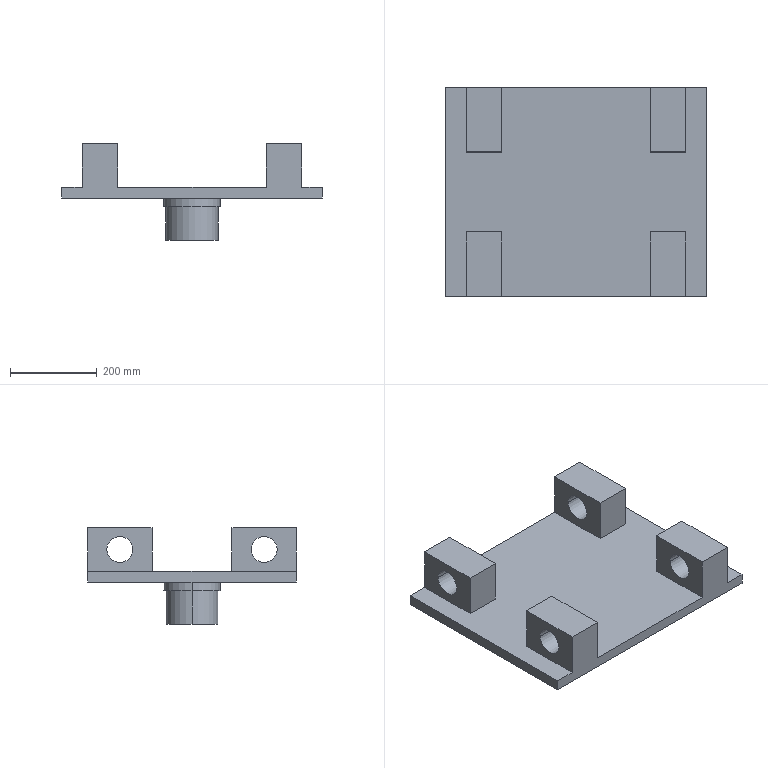Part | SolidWorks | features ICE 5, Extrusion 1 | 1 solid | 39 faces | box 600 x 480 x 222 mm | volume 11838573 mm3 | plane 25 | cylinder 14 | commonest cylinder face diameters 60 x8 80 x2 120 x2 130 x2
STEP:
#1=CARTESIAN_POINT('',(340.,240.,-97.));
#2=VERTEX_POINT('',#1);
#3=CARTESIAN_POINT('',(260.,240.,-97.));
#4=VERTEX_POINT('',#3);
#5=CARTESIAN_POINT('',(300.,240.,-97.));
#6=DIRECTION('',(0.,0.,-1.));
#7=DIRECTION('',(-1.,0.,0.));
#8=AXIS2_PLACEMENT_3D('',#5,#6,#7);
#9=CIRCLE('',#8,40.);
#10=EDGE_CURVE('',#2,#4,#9,.T.);
#11=ORIENTED_EDGE('',*,*,#10,.T.);
#12=CARTESIAN_POINT('',(260.,240.,-12.5));
#13=VERTEX_POINT('',#12);
#14=CARTESIAN_POINT('',(260.,240.,-20.));
#15=DIRECTION('',(0.,0.,1.));
#16=VECTOR('',#15,1000.);
#17=LINE('',#14,#16);
#18=EDGE_CURVE('',#4,#13,#17,.T.);
#19=ORIENTED_EDGE('',*,*,#18,.T.);
#20=CARTESIAN_POINT('',(340.,240.,-12.5));
#21=VERTEX_POINT('',#20);
#22=CARTESIAN_POINT('',(300.,240.,-12.5));
#23=DIRECTION('',(0.,0.,-1.));
#24=DIRECTION('',(-1.,0.,0.));
#25=AXIS2_PLACEMENT_3D('',#22,#23,#24);
#26=CIRCLE('',#25,40.);
#27=EDGE_CURVE('',#21,#13,#26,.T.);
#28=ORIENTED_EDGE('',*,*,#27,.F.);
#29=CARTESIAN_POINT('',(340.,240.,-20.));
#30=DIRECTION('',(0.,0.,1.));
#31=VECTOR('',#30,1000.);
#32=LINE('',#29,#31);
#33=EDGE_CURVE('',#2,#21,#32,.T.);
#34=ORIENTED_EDGE('',*,*,#33,.F.);
#35=EDGE_LOOP('',(#11,#19,#28,#34));
#36=FACE_OUTER_BOUND('',#35,.T.);
#37=CARTESIAN_POINT('',(300.,240.,-20.));
#38=DIRECTION('',(0.,0.,1.));
#39=DIRECTION('',(1.,0.,0.));
#40=AXIS2_PLACEMENT_3D('',#37,#38,#39);
#41=CYLINDRICAL_SURFACE('',#40,40.);
#42=ADVANCED_FACE('',(#36),#41,.F.);
#43=CARTESIAN_POINT('',(240.,240.,-97.));
#44=VERTEX_POINT('',#43);
#45=CARTESIAN_POINT('',(360.,240.,-97.));
#46=VERTEX_POINT('',#45);
#47=CARTESIAN_POINT('',(300.,240.,-97.));
#48=DIRECTION('',(0.,0.,-1.));
#49=DIRECTION('',(-1.,0.,0.));
#50=AXIS2_PLACEMENT_3D('',#47,#48,#49);
#51=CIRCLE('',#50,60.);
#52=EDGE_CURVE('',#44,#46,#51,.T.);
#53=ORIENTED_EDGE('',*,*,#52,.F.);
#54=CARTESIAN_POINT('',(240.,240.,-20.));
#55=VERTEX_POINT('',#54);
#56=CARTESIAN_POINT('',(240.,240.,-97.));
#57=DIRECTION('',(0.,0.,1.));
#58=VECTOR('',#57,1000.);
#59=LINE('',#56,#58);
#60=EDGE_CURVE('',#44,#55,#59,.T.);
#61=ORIENTED_EDGE('',*,*,#60,.T.);
#62=CARTESIAN_POINT('',(360.,240.,-20.));
#63=VERTEX_POINT('',#62);
#64=CARTESIAN_POINT('',(300.,240.,-20.));
#65=DIRECTION('',(0.,0.,-1.));
#66=DIRECTION('',(-1.,0.,0.));
#67=AXIS2_PLACEMENT_3D('',#64,#65,#66);
#68=CIRCLE('',#67,60.);
#69=EDGE_CURVE('',#55,#63,#68,.T.);
#70=ORIENTED_EDGE('',*,*,#69,.T.);
#71=CARTESIAN_POINT('',(360.,240.,-97.));
#72=DIRECTION('',(0.,0.,1.));
#73=VECTOR('',#72,1000.);
#74=LINE('',#71,#73);
#75=EDGE_CURVE('',#46,#63,#74,.T.);
#76=ORIENTED_EDGE('',*,*,#75,.F.);
#77=EDGE_LOOP('',(#53,#61,#70,#76));
#78=FACE_OUTER_BOUND('',#77,.T.);
#79=CARTESIAN_POINT('',(300.,240.,-97.));
#80=DIRECTION('',(0.,0.,1.));
#81=DIRECTION('',(1.,0.,0.));
#82=AXIS2_PLACEMENT_3D('',#79,#80,#81);
#83=CYLINDRICAL_SURFACE('',#82,60.);
#84=ADVANCED_FACE('',(#78),#83,.T.);
#85=CARTESIAN_POINT('',(235.,240.,-20.));
#86=VERTEX_POINT('',#85);
#87=CARTESIAN_POINT('',(365.,240.,-20.));
#88=VERTEX_POINT('',#87);
#89=CARTESIAN_POINT('',(300.,240.,-20.));
#90=DIRECTION('',(0.,0.,-1.));
#91=DIRECTION('',(-1.,0.,0.));
#92=AXIS2_PLACEMENT_3D('',#89,#90,#91);
#93=CIRCLE('',#92,65.);
#94=EDGE_CURVE('',#86,#88,#93,.T.);
#95=ORIENTED_EDGE('',*,*,#94,.F.);
#96=CARTESIAN_POINT('',(235.,240.,0.));
#97=VERTEX_POINT('',#96);
#98=CARTESIAN_POINT('',(235.,240.,-20.));
#99=DIRECTION('',(0.,0.,1.));
#100=VECTOR('',#99,1000.);
#101=LINE('',#98,#100);
#102=EDGE_CURVE('',#86,#97,#101,.T.);
#103=ORIENTED_EDGE('',*,*,#102,.T.);
#104=CARTESIAN_POINT('',(365.,240.,0.));
#105=VERTEX_POINT('',#104);
#106=CARTESIAN_POINT('',(300.,240.,0.));
#107=DIRECTION('',(0.,0.,-1.));
#108=DIRECTION('',(-1.,0.,0.));
#109=AXIS2_PLACEMENT_3D('',#106,#107,#108);
#110=CIRCLE('',#109,65.);
#111=EDGE_CURVE('',#97,#105,#110,.T.);
#112=ORIENTED_EDGE('',*,*,#111,.T.);
#113=CARTESIAN_POINT('',(365.,240.,-20.));
#114=DIRECTION('',(0.,0.,1.));
#115=VECTOR('',#114,1000.);
#116=LINE('',#113,#115);
#117=EDGE_CURVE('',#88,#105,#116,.T.);
#118=ORIENTED_EDGE('',*,*,#117,.F.);
#119=EDGE_LOOP('',(#95,#103,#112,#118));
#120=FACE_OUTER_BOUND('',#119,.T.);
#121=CARTESIAN_POINT('',(300.,240.,-20.));
#122=DIRECTION('',(0.,0.,1.));
#123=DIRECTION('',(1.,0.,0.));
#124=AXIS2_PLACEMENT_3D('',#121,#122,#123);
#125=CYLINDRICAL_SURFACE('',#124,65.);
#126=ADVANCED_FACE('',(#120),#125,.T.);
#127=CARTESIAN_POINT('',(129.5,44.,75.));
#128=VERTEX_POINT('',#127);
#129=CARTESIAN_POINT('',(129.5,104.,75.));
#130=VERTEX_POINT('',#129);
#131=CARTESIAN_POINT('',(129.5,74.,75.));
#132=DIRECTION('',(1.,0.,0.));
#133=DIRECTION('',(0.,0.,-1.));
#134=AXIS2_PLACEMENT_3D('',#131,#132,#133);
#135=CIRCLE('',#134,30.);
#136=EDGE_CURVE('',#128,#130,#135,.T.);
#137=ORIENTED_EDGE('',*,*,#136,.T.);
#138=CARTESIAN_POINT('',(47.5,104.,75.));
#139=VERTEX_POINT('',#138);
#140=CARTESIAN_POINT('',(600.,104.,75.));
#141=DIRECTION('',(-1.,0.,0.));
#142=VECTOR('',#141,1000.);
#143=LINE('',#140,#142);
#144=EDGE_CURVE('',#130,#139,#143,.T.);
#145=ORIENTED_EDGE('',*,*,#144,.T.);
#146=CARTESIAN_POINT('',(47.5,44.,75.));
#147=VERTEX_POINT('',#146);
#148=CARTESIAN_POINT('',(47.5,74.,75.));
#149=DIRECTION('',(-1.,0.,0.));
#150=DIRECTION('',(0.,-1.,0.));
#151=AXIS2_PLACEMENT_3D('',#148,#149,#150);
#152=CIRCLE('',#151,30.);
#153=EDGE_CURVE('',#139,#147,#152,.T.);
#154=ORIENTED_EDGE('',*,*,#153,.T.);
#155=CARTESIAN_POINT('',(600.,44.,75.));
#156=DIRECTION('',(-1.,0.,0.));
#157=VECTOR('',#156,1000.);
#158=LINE('',#155,#157);
#159=EDGE_CURVE('',#128,#147,#158,.T.);
#160=ORIENTED_EDGE('',*,*,#159,.F.);
#161=EDGE_LOOP('',(#137,#145,#154,#160));
#162=FACE_OUTER_BOUND('',#161,.T.);
#163=CARTESIAN_POINT('',(600.,74.,75.));
#164=DIRECTION('',(-1.,0.,0.));
#165=DIRECTION('',(0.,-1.,0.));
#166=AXIS2_PLACEMENT_3D('',#163,#164,#165);
#167=CYLINDRICAL_SURFACE('',#166,30.);
#168=ADVANCED_FACE('',(#162),#167,.F.);
#169=CARTESIAN_POINT('',(552.5,44.,75.));
#170=VERTEX_POINT('',#169);
#171=CARTESIAN_POINT('',(552.5,104.,75.));
#172=VERTEX_POINT('',#171);
#173=CARTESIAN_POINT('',(552.5,74.,75.));
#174=DIRECTION('',(1.,0.,0.));
#175=DIRECTION('',(0.,1.,0.));
#176=AXIS2_PLACEMENT_3D('',#173,#174,#175);
#177=CIRCLE('',#176,30.);
#178=EDGE_CURVE('',#170,#172,#177,.T.);
#179=ORIENTED_EDGE('',*,*,#178,.T.);
#180=CARTESIAN_POINT('',(470.5,104.,75.));
#181=VERTEX_POINT('',#180);
#182=CARTESIAN_POINT('',(600.,104.,75.));
#183=DIRECTION('',(-1.,0.,0.));
#184=VECTOR('',#183,1000.);
#185=LINE('',#182,#184);
#186=EDGE_CURVE('',#172,#181,#185,.T.);
#187=ORIENTED_EDGE('',*,*,#186,.T.);
#188=CARTESIAN_POINT('',(470.5,44.,75.));
#189=VERTEX_POINT('',#188);
#190=CARTESIAN_POINT('',(470.5,74.,75.));
#191=DIRECTION('',(1.,0.,0.));
#192=DIRECTION('',(0.,0.,-1.));
#193=AXIS2_PLACEMENT_3D('',#190,#191,#192);
#194=CIRCLE('',#193,30.);
#195=EDGE_CURVE('',#189,#181,#194,.T.);
#196=ORIENTED_EDGE('',*,*,#195,.F.);
#197=CARTESIAN_POINT('',(600.,44.,75.));
#198=DIRECTION('',(-1.,0.,0.));
#199=VECTOR('',#198,1000.);
#200=LINE('',#197,#199);
#201=EDGE_CURVE('',#170,#189,#200,.T.);
#202=ORIENTED_EDGE('',*,*,#201,.F.);
#203=EDGE_LOOP('',(#179,#187,#196,#202));
#204=FACE_OUTER_BOUND('',#203,.T.);
#205=CARTESIAN_POINT('',(600.,74.,75.));
#206=DIRECTION('',(-1.,0.,0.));
#207=DIRECTION('',(0.,-1.,0.));
#208=AXIS2_PLACEMENT_3D('',#205,#206,#207);
#209=CYLINDRICAL_SURFACE('',#208,30.);
#210=ADVANCED_FACE('',(#204),#209,.F.);
#211=CARTESIAN_POINT('',(129.5,376.,75.));
#212=VERTEX_POINT('',#211);
#213=CARTESIAN_POINT('',(129.5,436.,75.));
#214=VERTEX_POINT('',#213);
#215=CARTESIAN_POINT('',(129.5,406.,75.));
#216=DIRECTION('',(1.,0.,0.));
#217=DIRECTION('',(0.,1.,0.));
#218=AXIS2_PLACEMENT_3D('',#215,#216,#217);
#219=CIRCLE('',#218,30.);
#220=EDGE_CURVE('',#212,#214,#219,.T.);
#221=ORIENTED_EDGE('',*,*,#220,.T.);
#222=CARTESIAN_POINT('',(47.5,436.,75.));
#223=VERTEX_POINT('',#222);
#224=CARTESIAN_POINT('',(600.,436.,75.));
#225=DIRECTION('',(-1.,0.,0.));
#226=VECTOR('',#225,1000.);
#227=LINE('',#224,#226);
#228=EDGE_CURVE('',#214,#223,#227,.T.);
#229=ORIENTED_EDGE('',*,*,#228,.T.);
#230=CARTESIAN_POINT('',(47.5,376.,75.));
#231=VERTEX_POINT('',#230);
#232=CARTESIAN_POINT('',(47.5,406.,75.));
#233=DIRECTION('',(-1.,0.,0.));
#234=DIRECTION('',(0.,-1.,0.));
#235=AXIS2_PLACEMENT_3D('',#232,#233,#234);
#236=CIRCLE('',#235,30.);
#237=EDGE_CURVE('',#223,#231,#236,.T.);
#238=ORIENTED_EDGE('',*,*,#237,.T.);
#239=CARTESIAN_POINT('',(600.,376.,75.));
#240=DIRECTION('',(-1.,0.,0.));
#241=VECTOR('',#240,1000.);
#242=LINE('',#239,#241);
#243=EDGE_CURVE('',#212,#231,#242,.T.);
#244=ORIENTED_EDGE('',*,*,#243,.F.);
#245=EDGE_LOOP('',(#221,#229,#238,#244));
#246=FACE_OUTER_BOUND('',#245,.T.);
#247=CARTESIAN_POINT('',(600.,406.,75.));
#248=DIRECTION('',(-1.,0.,0.));
#249=DIRECTION('',(0.,-1.,0.));
#250=AXIS2_PLACEMENT_3D('',#247,#248,#249);
#251=CYLINDRICAL_SURFACE('',#250,30.);
#252=ADVANCED_FACE('',(#246),#251,.F.);
#253=CARTESIAN_POINT('',(552.5,376.,75.));
#254=VERTEX_POINT('',#253);
#255=CARTESIAN_POINT('',(552.5,436.,75.));
#256=VERTEX_POINT('',#255);
#257=CARTESIAN_POINT('',(552.5,406.,75.));
#258=DIRECTION('',(1.,0.,0.));
#259=DIRECTION('',(0.,0.,-1.));
#260=AXIS2_PLACEMENT_3D('',#257,#258,#259);
#261=CIRCLE('',#260,30.);
#262=EDGE_CURVE('',#254,#256,#261,.T.);
#263=ORIENTED_EDGE('',*,*,#262,.T.);
#264=CARTESIAN_POINT('',(470.5,436.,75.));
#265=VERTEX_POINT('',#264);
#266=CARTESIAN_POINT('',(600.,436.,75.));
#267=DIRECTION('',(-1.,0.,0.));
#268=VECTOR('',#267,1000.);
#269=LINE('',#266,#268);
#270=EDGE_CURVE('',#256,#265,#269,.T.);
#271=ORIENTED_EDGE('',*,*,#270,.T.);
#272=CARTESIAN_POINT('',(470.5,376.,75.));
#273=VERTEX_POINT('',#272);
#274=CARTESIAN_POINT('',(470.5,406.,75.));
#275=DIRECTION('',(1.,0.,0.));
#276=DIRECTION('',(0.,0.,-1.));
#277=AXIS2_PLACEMENT_3D('',#274,#275,#276);
#278=CIRCLE('',#277,30.);
#279=EDGE_CURVE('',#273,#265,#278,.T.);
#280=ORIENTED_EDGE('',*,*,#279,.F.);
#281=CARTESIAN_POINT('',(600.,376.,75.));
#282=DIRECTION('',(-1.,0.,0.));
#283=VECTOR('',#282,1000.);
#284=LINE('',#281,#283);
#285=EDGE_CURVE('',#254,#273,#284,.T.);
#286=ORIENTED_EDGE('',*,*,#285,.F.);
#287=EDGE_LOOP('',(#263,#271,#280,#286));
#288=FACE_OUTER_BOUND('',#287,.T.);
#289=CARTESIAN_POINT('',(600.,406.,75.));
#290=DIRECTION('',(-1.,0.,0.));
#291=DIRECTION('',(0.,-1.,0.));
#292=AXIS2_PLACEMENT_3D('',#289,#290,#291);
#293=CYLINDRICAL_SURFACE('',#292,30.);
#294=ADVANCED_FACE('',(#288),#293,.F.);
#295=CARTESIAN_POINT('',(300.,240.,-20.));
#296=DIRECTION('',(0.,0.,-1.));
#297=DIRECTION('',(-1.,0.,0.));
#298=AXIS2_PLACEMENT_3D('',#295,#296,#297);
#299=CIRCLE('',#298,65.);
#300=EDGE_CURVE('',#88,#86,#299,.T.);
#301=ORIENTED_EDGE('',*,*,#300,.T.);
#302=ORIENTED_EDGE('',*,*,#94,.T.);
#303=EDGE_LOOP('',(#301,#302));
#304=FACE_OUTER_BOUND('',#303,.T.);
#305=CARTESIAN_POINT('',(300.,240.,-20.));
#306=DIRECTION('',(0.,0.,-1.));
#307=DIRECTION('',(-1.,0.,0.));
#308=AXIS2_PLACEMENT_3D('',#305,#306,#307);
#309=CIRCLE('',#308,60.);
#310=EDGE_CURVE('',#63,#55,#309,.T.);
#311=ORIENTED_EDGE('',*,*,#310,.F.);
#312=ORIENTED_EDGE('',*,*,#69,.F.);
#313=EDGE_LOOP('',(#311,#312));
#314=FACE_BOUND('',#313,.T.);
#315=CARTESIAN_POINT('',(300.,240.,-20.));
#316=DIRECTION('',(0.,0.,-1.));
#317=DIRECTION('',(-1.,0.,0.));
#318=AXIS2_PLACEMENT_3D('',#315,#316,#317);
#319=PLANE('',#318);
#320=ADVANCED_FACE('',(#304,#314),#319,.T.);
#321=CARTESIAN_POINT('',(0.,0.,0.));
#322=VERTEX_POINT('',#321);
#323=CARTESIAN_POINT('',(600.,0.,0.));
#324=VERTEX_POINT('',#323);
#325=CARTESIAN_POINT('',(600.,0.,0.));
#326=DIRECTION('',(1.,0.,0.));
#327=VECTOR('',#326,1000.);
#328=LINE('',#325,#327);
#329=EDGE_CURVE('',#322,#324,#328,.T.);
#330=ORIENTED_EDGE('',*,*,#329,.F.);
#331=CARTESIAN_POINT('',(0.,480.,0.));
#332=VERTEX_POINT('',#331);
#333=CARTESIAN_POINT('',(0.,0.,0.));
#334=DIRECTION('',(0.,-1.,0.));
#335=VECTOR('',#334,1000.);
#336=LINE('',#333,#335);
#337=EDGE_CURVE('',#332,#322,#336,.T.);
#338=ORIENTED_EDGE('',*,*,#337,.F.);
#339=CARTESIAN_POINT('',(600.,480.,0.));
#340=VERTEX_POINT('',#339);
#341=CARTESIAN_POINT('',(0.,480.,0.));
#342=DIRECTION('',(-1.,0.,0.));
#343=VECTOR('',#342,1000.);
#344=LINE('',#341,#343);
#345=EDGE_CURVE('',#340,#332,#344,.T.);
#346=ORIENTED_EDGE('',*,*,#345,.F.);
#347=CARTESIAN_POINT('',(600.,480.,0.));
#348=DIRECTION('',(0.,1.,0.));
#349=VECTOR('',#348,1000.);
#350=LINE('',#347,#349);
#351=EDGE_CURVE('',#324,#340,#350,.T.);
#352=ORIENTED_EDGE('',*,*,#351,.F.);
#353=EDGE_LOOP('',(#330,#338,#346,#352));
#354=FACE_OUTER_BOUND('',#353,.T.);
#355=CARTESIAN_POINT('',(300.,240.,0.));
#356=DIRECTION('',(0.,0.,-1.));
#357=DIRECTION('',(-1.,0.,0.));
#358=AXIS2_PLACEMENT_3D('',#355,#356,#357);
#359=CIRCLE('',#358,65.);
#360=EDGE_CURVE('',#105,#97,#359,.T.);
#361=ORIENTED_EDGE('',*,*,#360,.F.);
#362=ORIENTED_EDGE('',*,*,#111,.F.);
#363=EDGE_LOOP('',(#361,#362));
#364=FACE_BOUND('',#363,.T.);
#365=CARTESIAN_POINT('',(0.,0.,0.));
#366=DIRECTION('',(0.,0.,-1.));
#367=DIRECTION('',(-1.,0.,0.));
#368=AXIS2_PLACEMENT_3D('',#365,#366,#367);
#369=PLANE('',#368);
#370=ADVANCED_FACE('',(#354,#364),#369,.T.);
#371=CARTESIAN_POINT('',(470.5,480.,25.));
#372=VERTEX_POINT('',#371);
#373=CARTESIAN_POINT('',(470.5,332.,25.));
#374=VERTEX_POINT('',#373);
#375=CARTESIAN_POINT('',(470.5,-357.797,25.));
#376=DIRECTION('',(0.,-1.,0.));
#377=VECTOR('',#376,1000.);
#378=LINE('',#375,#377);
#379=EDGE_CURVE('',#372,#374,#378,.T.);
#380=ORIENTED_EDGE('',*,*,#379,.F.);
#381=CARTESIAN_POINT('',(129.5,480.,25.));
#382=VERTEX_POINT('',#381);
#383=CARTESIAN_POINT('',(0.,480.,25.));
#384=DIRECTION('',(-1.,0.,0.));
#385=VECTOR('',#384,1000.);
#386=LINE('',#383,#385);
#387=EDGE_CURVE('',#372,#382,#386,.T.);
#388=ORIENTED_EDGE('',*,*,#387,.T.);
#389=CARTESIAN_POINT('',(129.5,332.,25.));
#390=VERTEX_POINT('',#389);
#391=CARTESIAN_POINT('',(129.5,-357.797,25.));
#392=DIRECTION('',(0.,-1.,0.));
#393=VECTOR('',#392,1000.);
#394=LINE('',#391,#393);
#395=EDGE_CURVE('',#382,#390,#394,.T.);
#396=ORIENTED_EDGE('',*,*,#395,.T.);
#397=CARTESIAN_POINT('',(47.5,332.,25.));
#398=VERTEX_POINT('',#397);
#399=CARTESIAN_POINT('',(300.,332.,25.));
#400=DIRECTION('',(1.,0.,0.));
#401=VECTOR('',#400,1000.);
#402=LINE('',#399,#401);
#403=EDGE_CURVE('',#398,#390,#402,.T.);
#404=ORIENTED_EDGE('',*,*,#403,.F.);
#405=CARTESIAN_POINT('',(47.5,480.,25.));
#406=VERTEX_POINT('',#405);
#407=CARTESIAN_POINT('',(47.5,-357.797,25.));
#408=DIRECTION('',(0.,-1.,0.));
#409=VECTOR('',#408,1000.);
#410=LINE('',#407,#409);
#411=EDGE_CURVE('',#406,#398,#410,.T.);
#412=ORIENTED_EDGE('',*,*,#411,.F.);
#413=CARTESIAN_POINT('',(0.,480.,25.));
#414=VERTEX_POINT('',#413);
#415=CARTESIAN_POINT('',(0.,480.,25.));
#416=DIRECTION('',(-1.,0.,0.));
#417=VECTOR('',#416,1000.);
#418=LINE('',#415,#417);
#419=EDGE_CURVE('',#406,#414,#418,.T.);
#420=ORIENTED_EDGE('',*,*,#419,.T.);
#421=CARTESIAN_POINT('',(0.,0.,25.));
#422=VERTEX_POINT('',#421);
#423=CARTESIAN_POINT('',(0.,0.,25.));
#424=DIRECTION('',(0.,-1.,0.));
#425=VECTOR('',#424,1000.);
#426=LINE('',#423,#425);
#427=EDGE_CURVE('',#414,#422,#426,.T.);
#428=ORIENTED_EDGE('',*,*,#427,.T.);
#429=CARTESIAN_POINT('',(47.5,0.,25.));
#430=VERTEX_POINT('',#429);
#431=CARTESIAN_POINT('',(600.,0.,25.));
#432=DIRECTION('',(1.,0.,0.));
#433=VECTOR('',#432,1000.);
#434=LINE('',#431,#433);
#435=EDGE_CURVE('',#422,#430,#434,.T.);
#436=ORIENTED_EDGE('',*,*,#435,.T.);
#437=CARTESIAN_POINT('',(47.5,148.,25.));
#438=VERTEX_POINT('',#437);
#439=CARTESIAN_POINT('',(47.5,-357.797,25.));
#440=DIRECTION('',(0.,-1.,0.));
#441=VECTOR('',#440,1000.);
#442=LINE('',#439,#441);
#443=EDGE_CURVE('',#438,#430,#442,.T.);
#444=ORIENTED_EDGE('',*,*,#443,.F.);
#445=CARTESIAN_POINT('',(129.5,148.,25.));
#446=VERTEX_POINT('',#445);
#447=CARTESIAN_POINT('',(300.,148.,25.));
#448=DIRECTION('',(1.,0.,0.));
#449=VECTOR('',#448,1000.);
#450=LINE('',#447,#449);
#451=EDGE_CURVE('',#438,#446,#450,.T.);
#452=ORIENTED_EDGE('',*,*,#451,.T.);
#453=CARTESIAN_POINT('',(129.5,0.,25.));
#454=VERTEX_POINT('',#453);
#455=CARTESIAN_POINT('',(129.5,-357.797,25.));
#456=DIRECTION('',(0.,-1.,0.));
#457=VECTOR('',#456,1000.);
#458=LINE('',#455,#457);
#459=EDGE_CURVE('',#446,#454,#458,.T.);
#460=ORIENTED_EDGE('',*,*,#459,.T.);
#461=CARTESIAN_POINT('',(470.5,0.,25.));
#462=VERTEX_POINT('',#461);
#463=CARTESIAN_POINT('',(600.,0.,25.));
#464=DIRECTION('',(1.,0.,0.));
#465=VECTOR('',#464,1000.);
#466=LINE('',#463,#465);
#467=EDGE_CURVE('',#454,#462,#466,.T.);
#468=ORIENTED_EDGE('',*,*,#467,.T.);
#469=CARTESIAN_POINT('',(470.5,148.,25.));
#470=VERTEX_POINT('',#469);
#471=CARTESIAN_POINT('',(470.5,-357.797,25.));
#472=DIRECTION('',(0.,-1.,0.));
#473=VECTOR('',#472,1000.);
#474=LINE('',#471,#473);
#475=EDGE_CURVE('',#470,#462,#474,.T.);
#476=ORIENTED_EDGE('',*,*,#475,.F.);
#477=CARTESIAN_POINT('',(552.5,148.,25.));
#478=VERTEX_POINT('',#477);
#479=CARTESIAN_POINT('',(300.,148.,25.));
#480=DIRECTION('',(1.,0.,0.));
#481=VECTOR('',#480,1000.);
#482=LINE('',#479,#481);
#483=EDGE_CURVE('',#470,#478,#482,.T.);
#484=ORIENTED_EDGE('',*,*,#483,.T.);
#485=CARTESIAN_POINT('',(552.5,0.,25.));
#486=VERTEX_POINT('',#485);
#487=CARTESIAN_POINT('',(552.5,-357.797,25.));
#488=DIRECTION('',(0.,-1.,0.));
#489=VECTOR('',#488,1000.);
#490=LINE('',#487,#489);
#491=EDGE_CURVE('',#478,#486,#490,.T.);
#492=ORIENTED_EDGE('',*,*,#491,.T.);
#493=CARTESIAN_POINT('',(600.,0.,25.));
#494=VERTEX_POINT('',#493);
#495=CARTESIAN_POINT('',(600.,0.,25.));
#496=DIRECTION('',(1.,0.,0.));
#497=VECTOR('',#496,1000.);
#498=LINE('',#495,#497);
#499=EDGE_CURVE('',#486,#494,#498,.T.);
#500=ORIENTED_EDGE('',*,*,#499,.T.);
#501=CARTESIAN_POINT('',(600.,480.,25.));
#502=VERTEX_POINT('',#501);
#503=CARTESIAN_POINT('',(600.,480.,25.));
#504=DIRECTION('',(0.,1.,0.));
#505=VECTOR('',#504,1000.);
#506=LINE('',#503,#505);
#507=EDGE_CURVE('',#494,#502,#506,.T.);
#508=ORIENTED_EDGE('',*,*,#507,.T.);
#509=CARTESIAN_POINT('',(552.5,480.,25.));
#510=VERTEX_POINT('',#509);
#511=CARTESIAN_POINT('',(0.,480.,25.));
#512=DIRECTION('',(-1.,0.,0.));
#513=VECTOR('',#512,1000.);
#514=LINE('',#511,#513);
#515=EDGE_CURVE('',#502,#510,#514,.T.);
#516=ORIENTED_EDGE('',*,*,#515,.T.);
#517=CARTESIAN_POINT('',(552.5,332.,25.));
#518=VERTEX_POINT('',#517);
#519=CARTESIAN_POINT('',(552.5,-357.797,25.));
#520=DIRECTION('',(0.,-1.,0.));
#521=VECTOR('',#520,1000.);
#522=LINE('',#519,#521);
#523=EDGE_CURVE('',#510,#518,#522,.T.);
#524=ORIENTED_EDGE('',*,*,#523,.T.);
#525=CARTESIAN_POINT('',(300.,332.,25.));
#526=DIRECTION('',(1.,0.,0.));
#527=VECTOR('',#526,1000.);
#528=LINE('',#525,#527);
#529=EDGE_CURVE('',#374,#518,#528,.T.);
#530=ORIENTED_EDGE('',*,*,#529,.F.);
#531=EDGE_LOOP('',(#380,#388,#396,#404,#412,#420,#428,#436,#444,#452,#460,#468,#476,#484,#492,#500,#508,#516,#524,#530));
#532=FACE_OUTER_BOUND('',#531,.T.);
#533=CARTESIAN_POINT('',(0.,0.,25.));
#534=DIRECTION('',(0.,0.,-1.));
#535=DIRECTION('',(-1.,0.,0.));
#536=AXIS2_PLACEMENT_3D('',#533,#534,#535);
#537=PLANE('',#536);
#538=ADVANCED_FACE('',(#532),#537,.F.);
#539=ORIENTED_EDGE('',*,*,#329,.T.);
#540=CARTESIAN_POINT('',(600.,0.,25.));
#541=DIRECTION('',(0.,0.,-1.));
#542=VECTOR('',#541,1000.);
#543=LINE('',#540,#542);
#544=EDGE_CURVE('',#494,#324,#543,.T.);
#545=ORIENTED_EDGE('',*,*,#544,.F.);
#546=ORIENTED_EDGE('',*,*,#499,.F.);
#547=CARTESIAN_POINT('',(552.5,0.,125.));
#548=VERTEX_POINT('',#547);
#549=CARTESIAN_POINT('',(552.5,0.,125.));
#550=DIRECTION('',(0.,0.,-1.));
#551=VECTOR('',#550,1000.);
#552=LINE('',#549,#551);
#553=EDGE_CURVE('',#548,#486,#552,.T.);
#554=ORIENTED_EDGE('',*,*,#553,.F.);
#555=CARTESIAN_POINT('',(470.5,0.,125.));
#556=VERTEX_POINT('',#555);
#557=CARTESIAN_POINT('',(300.,0.,125.));
#558=DIRECTION('',(1.,0.,0.));
#559=VECTOR('',#558,1000.);
#560=LINE('',#557,#559);
#561=EDGE_CURVE('',#556,#548,#560,.T.);
#562=ORIENTED_EDGE('',*,*,#561,.F.);
#563=CARTESIAN_POINT('',(470.5,0.,125.));
#564=DIRECTION('',(0.,0.,-1.));
#565=VECTOR('',#564,1000.);
#566=LINE('',#563,#565);
#567=EDGE_CURVE('',#556,#462,#566,.T.);
#568=ORIENTED_EDGE('',*,*,#567,.T.);
#569=ORIENTED_EDGE('',*,*,#467,.F.);
#570=CARTESIAN_POINT('',(129.5,0.,125.));
#571=VERTEX_POINT('',#570);
#572=CARTESIAN_POINT('',(129.5,0.,125.));
#573=DIRECTION('',(0.,0.,-1.));
#574=VECTOR('',#573,1000.);
#575=LINE('',#572,#574);
#576=EDGE_CURVE('',#571,#454,#575,.T.);
#577=ORIENTED_EDGE('',*,*,#576,.F.);
#578=CARTESIAN_POINT('',(47.5,0.,125.));
#579=VERTEX_POINT('',#578);
#580=CARTESIAN_POINT('',(300.,0.,125.));
#581=DIRECTION('',(1.,0.,0.));
#582=VECTOR('',#581,1000.);
#583=LINE('',#580,#582);
#584=EDGE_CURVE('',#579,#571,#583,.T.);
#585=ORIENTED_EDGE('',*,*,#584,.F.);
#586=CARTESIAN_POINT('',(47.5,0.,125.));
#587=DIRECTION('',(0.,0.,-1.));
#588=VECTOR('',#587,1000.);
#589=LINE('',#586,#588);
#590=EDGE_CURVE('',#579,#430,#589,.T.);
#591=ORIENTED_EDGE('',*,*,#590,.T.);
#592=ORIENTED_EDGE('',*,*,#435,.F.);
#593=CARTESIAN_POINT('',(0.,0.,25.));
#594=DIRECTION('',(0.,0.,-1.));
#595=VECTOR('',#594,1000.);
#596=LINE('',#593,#595);
#597=EDGE_CURVE('',#422,#322,#596,.T.);
#598=ORIENTED_EDGE('',*,*,#597,.T.);
#599=EDGE_LOOP('',(#539,#545,#546,#554,#562,#568,#569,#577,#585,#591,#592,#598));
#600=FACE_OUTER_BOUND('',#599,.T.);
#601=CARTESIAN_POINT('',(600.,0.,25.));
#602=DIRECTION('',(0.,1.,0.));
#603=DIRECTION('',(-1.,0.,0.));
#604=AXIS2_PLACEMENT_3D('',#601,#602,#603);
#605=PLANE('',#604);
#606=ADVANCED_FACE('',(#600),#605,.F.);
#607=ORIENTED_EDGE('',*,*,#351,.T.);
#608=CARTESIAN_POINT('',(600.,480.,25.));
#609=DIRECTION('',(0.,0.,-1.));
#610=VECTOR('',#609,1000.);
#611=LINE('',#608,#610);
#612=EDGE_CURVE('',#502,#340,#611,.T.);
#613=ORIENTED_EDGE('',*,*,#612,.F.);
#614=ORIENTED_EDGE('',*,*,#507,.F.);
#615=ORIENTED_EDGE('',*,*,#544,.T.);
#616=EDGE_LOOP('',(#607,#613,#614,#615));
#617=FACE_OUTER_BOUND('',#616,.T.);
#618=CARTESIAN_POINT('',(600.,480.,25.));
#619=DIRECTION('',(-1.,0.,0.));
#620=DIRECTION('',(0.,-1.,0.));
#621=AXIS2_PLACEMENT_3D('',#618,#619,#620);
#622=PLANE('',#621);
#623=ADVANCED_FACE('',(#617),#622,.F.);
#624=ORIENTED_EDGE('',*,*,#345,.T.);
#625=CARTESIAN_POINT('',(0.,480.,25.));
#626=DIRECTION('',(0.,0.,-1.));
#627=VECTOR('',#626,1000.);
#628=LINE('',#625,#627);
#629=EDGE_CURVE('',#414,#332,#628,.T.);
#630=ORIENTED_EDGE('',*,*,#629,.F.);
#631=ORIENTED_EDGE('',*,*,#419,.F.);
#632=CARTESIAN_POINT('',(47.5,480.,125.));
#633=VERTEX_POINT('',#632);
#634=CARTESIAN_POINT('',(47.5,480.,125.));
#635=DIRECTION('',(0.,0.,-1.));
#636=VECTOR('',#635,1000.);
#637=LINE('',#634,#636);
#638=EDGE_CURVE('',#633,#406,#637,.T.);
#639=ORIENTED_EDGE('',*,*,#638,.F.);
#640=CARTESIAN_POINT('',(129.5,480.,125.));
#641=VERTEX_POINT('',#640);
#642=CARTESIAN_POINT('',(300.,480.,125.));
#643=DIRECTION('',(-1.,0.,0.));
#644=VECTOR('',#643,1000.);
#645=LINE('',#642,#644);
#646=EDGE_CURVE('',#641,#633,#645,.T.);
#647=ORIENTED_EDGE('',*,*,#646,.F.);
#648=CARTESIAN_POINT('',(129.5,480.,125.));
#649=DIRECTION('',(0.,0.,-1.));
#650=VECTOR('',#649,1000.);
#651=LINE('',#648,#650);
#652=EDGE_CURVE('',#641,#382,#651,.T.);
#653=ORIENTED_EDGE('',*,*,#652,.T.);
#654=ORIENTED_EDGE('',*,*,#387,.F.);
#655=CARTESIAN_POINT('',(470.5,480.,125.));
#656=VERTEX_POINT('',#655);
#657=CARTESIAN_POINT('',(470.5,480.,125.));
#658=DIRECTION('',(0.,0.,-1.));
#659=VECTOR('',#658,1000.);
#660=LINE('',#657,#659);
#661=EDGE_CURVE('',#656,#372,#660,.T.);
#662=ORIENTED_EDGE('',*,*,#661,.F.);
#663=CARTESIAN_POINT('',(552.5,480.,125.));
#664=VERTEX_POINT('',#663);
#665=CARTESIAN_POINT('',(300.,480.,125.));
#666=DIRECTION('',(-1.,0.,0.));
#667=VECTOR('',#666,1000.);
#668=LINE('',#665,#667);
#669=EDGE_CURVE('',#664,#656,#668,.T.);
#670=ORIENTED_EDGE('',*,*,#669,.F.);
#671=CARTESIAN_POINT('',(552.5,480.,125.));
#672=DIRECTION('',(0.,0.,-1.));
#673=VECTOR('',#672,1000.);
#674=LINE('',#671,#673);
#675=EDGE_CURVE('',#664,#510,#674,.T.);
#676=ORIENTED_EDGE('',*,*,#675,.T.);
#677=ORIENTED_EDGE('',*,*,#515,.F.);
#678=ORIENTED_EDGE('',*,*,#612,.T.);
#679=EDGE_LOOP('',(#624,#630,#631,#639,#647,#653,#654,#662,#670,#676,#677,#678));
#680=FACE_OUTER_BOUND('',#679,.T.);
#681=CARTESIAN_POINT('',(0.,480.,25.));
#682=DIRECTION('',(0.,-1.,0.));
#683=DIRECTION('',(0.,0.,-1.));
#684=AXIS2_PLACEMENT_3D('',#681,#682,#683);
#685=PLANE('',#684);
#686=ADVANCED_FACE('',(#680),#685,.F.);
#687=ORIENTED_EDGE('',*,*,#337,.T.);
#688=ORIENTED_EDGE('',*,*,#597,.F.);
#689=ORIENTED_EDGE('',*,*,#427,.F.);
#690=ORIENTED_EDGE('',*,*,#629,.T.);
#691=EDGE_LOOP('',(#687,#688,#689,#690));
#692=FACE_OUTER_BOUND('',#691,.T.);
#693=CARTESIAN_POINT('',(0.,0.,25.));
#694=DIRECTION('',(1.,0.,0.));
#695=DIRECTION('',(0.,0.,-1.));
#696=AXIS2_PLACEMENT_3D('',#693,#694,#695);
#697=PLANE('',#696);
#698=ADVANCED_FACE('',(#692),#697,.F.);
#699=ORIENTED_EDGE('',*,*,#220,.F.);
#700=CARTESIAN_POINT('',(129.5,406.,75.));
#701=DIRECTION('',(1.,0.,0.));
#702=DIRECTION('',(0.,1.,0.));
#703=AXIS2_PLACEMENT_3D('',#700,#701,#702);
#704=CIRCLE('',#703,30.);
#705=EDGE_CURVE('',#214,#212,#704,.T.);
#706=ORIENTED_EDGE('',*,*,#705,.F.);
#707=EDGE_LOOP('',(#699,#706));
#708=FACE_BOUND('',#707,.T.);
#709=ORIENTED_EDGE('',*,*,#395,.F.);
#710=ORIENTED_EDGE('',*,*,#652,.F.);
#711=CARTESIAN_POINT('',(129.5,332.,125.));
#712=VERTEX_POINT('',#711);
#713=CARTESIAN_POINT('',(129.5,-357.797,125.));
#714=DIRECTION('',(0.,-1.,0.));
#715=VECTOR('',#714,1000.);
#716=LINE('',#713,#715);
#717=EDGE_CURVE('',#641,#712,#716,.T.);
#718=ORIENTED_EDGE('',*,*,#717,.T.);
#719=CARTESIAN_POINT('',(129.5,332.,125.));
#720=DIRECTION('',(0.,0.,-1.));
#721=VECTOR('',#720,1000.);
#722=LINE('',#719,#721);
#723=EDGE_CURVE('',#712,#390,#722,.T.);
#724=ORIENTED_EDGE('',*,*,#723,.T.);
#725=EDGE_LOOP('',(#709,#710,#718,#724));
#726=FACE_OUTER_BOUND('',#725,.T.);
#727=CARTESIAN_POINT('',(129.5,-357.797,125.));
#728=DIRECTION('',(1.,0.,0.));
#729=DIRECTION('',(0.,1.,0.));
#730=AXIS2_PLACEMENT_3D('',#727,#728,#729);
#731=PLANE('',#730);
#732=ADVANCED_FACE('',(#708,#726),#731,.T.);
#733=CARTESIAN_POINT('',(47.5,406.,75.));
#734=DIRECTION('',(-1.,0.,0.));
#735=DIRECTION('',(0.,-1.,0.));
#736=AXIS2_PLACEMENT_3D('',#733,#734,#735);
#737=CIRCLE('',#736,30.);
#738=EDGE_CURVE('',#231,#223,#737,.T.);
#739=ORIENTED_EDGE('',*,*,#738,.F.);
#740=ORIENTED_EDGE('',*,*,#237,.F.);
#741=EDGE_LOOP('',(#739,#740));
#742=FACE_BOUND('',#741,.T.);
#743=ORIENTED_EDGE('',*,*,#411,.T.);
#744=CARTESIAN_POINT('',(47.5,332.,125.));
#745=VERTEX_POINT('',#744);
#746=CARTESIAN_POINT('',(47.5,332.,125.));
#747=DIRECTION('',(0.,0.,-1.));
#748=VECTOR('',#747,1000.);
#749=LINE('',#746,#748);
#750=EDGE_CURVE('',#745,#398,#749,.T.);
#751=ORIENTED_EDGE('',*,*,#750,.F.);
#752=CARTESIAN_POINT('',(47.5,-357.797,125.));
#753=DIRECTION('',(0.,-1.,0.));
#754=VECTOR('',#753,1000.);
#755=LINE('',#752,#754);
#756=EDGE_CURVE('',#633,#745,#755,.T.);
#757=ORIENTED_EDGE('',*,*,#756,.F.);
#758=ORIENTED_EDGE('',*,*,#638,.T.);
#759=EDGE_LOOP('',(#743,#751,#757,#758));
#760=FACE_OUTER_BOUND('',#759,.T.);
#761=CARTESIAN_POINT('',(47.5,-357.797,125.));
#762=DIRECTION('',(1.,0.,0.));
#763=DIRECTION('',(0.,1.,0.));
#764=AXIS2_PLACEMENT_3D('',#761,#762,#763);
#765=PLANE('',#764);
#766=ADVANCED_FACE('',(#742,#760),#765,.F.);
#767=ORIENTED_EDGE('',*,*,#403,.T.);
#768=ORIENTED_EDGE('',*,*,#723,.F.);
#769=CARTESIAN_POINT('',(300.,332.,125.));
#770=DIRECTION('',(1.,0.,0.));
#771=VECTOR('',#770,1000.);
#772=LINE('',#769,#771);
#773=EDGE_CURVE('',#745,#712,#772,.T.);
#774=ORIENTED_EDGE('',*,*,#773,.F.);
#775=ORIENTED_EDGE('',*,*,#750,.T.);
#776=EDGE_LOOP('',(#767,#768,#774,#775));
#777=FACE_OUTER_BOUND('',#776,.T.);
#778=CARTESIAN_POINT('',(300.,332.,125.));
#779=DIRECTION('',(0.,1.,0.));
#780=DIRECTION('',(0.,0.,1.));
#781=AXIS2_PLACEMENT_3D('',#778,#779,#780);
#782=PLANE('',#781);
#783=ADVANCED_FACE('',(#777),#782,.F.);
#784=ORIENTED_EDGE('',*,*,#717,.F.);
#785=ORIENTED_EDGE('',*,*,#646,.T.);
#786=ORIENTED_EDGE('',*,*,#756,.T.);
#787=ORIENTED_EDGE('',*,*,#773,.T.);
#788=EDGE_LOOP('',(#784,#785,#786,#787));
#789=FACE_OUTER_BOUND('',#788,.T.);
#790=CARTESIAN_POINT('',(300.,-357.797,125.));
#791=DIRECTION('',(0.,0.,1.));
#792=DIRECTION('',(1.,0.,0.));
#793=AXIS2_PLACEMENT_3D('',#790,#791,#792);
#794=PLANE('',#793);
#795=ADVANCED_FACE('',(#789),#794,.T.);
#796=ORIENTED_EDGE('',*,*,#136,.F.);
#797=CARTESIAN_POINT('',(129.5,74.,75.));
#798=DIRECTION('',(1.,0.,0.));
#799=DIRECTION('',(0.,0.,-1.));
#800=AXIS2_PLACEMENT_3D('',#797,#798,#799);
#801=CIRCLE('',#800,30.);
#802=EDGE_CURVE('',#130,#128,#801,.T.);
#803=ORIENTED_EDGE('',*,*,#802,.F.);
#804=EDGE_LOOP('',(#796,#803));
#805=FACE_BOUND('',#804,.T.);
#806=ORIENTED_EDGE('',*,*,#459,.F.);
#807=CARTESIAN_POINT('',(129.5,148.,125.));
#808=VERTEX_POINT('',#807);
#809=CARTESIAN_POINT('',(129.5,148.,125.));
#810=DIRECTION('',(0.,0.,-1.));
#811=VECTOR('',#810,1000.);
#812=LINE('',#809,#811);
#813=EDGE_CURVE('',#808,#446,#812,.T.);
#814=ORIENTED_EDGE('',*,*,#813,.F.);
#815=CARTESIAN_POINT('',(129.5,-357.797,125.));
#816=DIRECTION('',(0.,-1.,0.));
#817=VECTOR('',#816,1000.);
#818=LINE('',#815,#817);
#819=EDGE_CURVE('',#808,#571,#818,.T.);
#820=ORIENTED_EDGE('',*,*,#819,.T.);
#821=ORIENTED_EDGE('',*,*,#576,.T.);
#822=EDGE_LOOP('',(#806,#814,#820,#821));
#823=FACE_OUTER_BOUND('',#822,.T.);
#824=CARTESIAN_POINT('',(129.5,-357.797,125.));
#825=DIRECTION('',(1.,0.,0.));
#826=DIRECTION('',(0.,0.,-1.));
#827=AXIS2_PLACEMENT_3D('',#824,#825,#826);
#828=PLANE('',#827);
#829=ADVANCED_FACE('',(#805,#823),#828,.T.);
#830=ORIENTED_EDGE('',*,*,#451,.F.);
#831=CARTESIAN_POINT('',(47.5,148.,125.));
#832=VERTEX_POINT('',#831);
#833=CARTESIAN_POINT('',(47.5,148.,125.));
#834=DIRECTION('',(0.,0.,-1.));
#835=VECTOR('',#834,1000.);
#836=LINE('',#833,#835);
#837=EDGE_CURVE('',#832,#438,#836,.T.);
#838=ORIENTED_EDGE('',*,*,#837,.F.);
#839=CARTESIAN_POINT('',(300.,148.,125.));
#840=DIRECTION('',(1.,0.,0.));
#841=VECTOR('',#840,1000.);
#842=LINE('',#839,#841);
#843=EDGE_CURVE('',#832,#808,#842,.T.);
#844=ORIENTED_EDGE('',*,*,#843,.T.);
#845=ORIENTED_EDGE('',*,*,#813,.T.);
#846=EDGE_LOOP('',(#830,#838,#844,#845));
#847=FACE_OUTER_BOUND('',#846,.T.);
#848=CARTESIAN_POINT('',(300.,148.,125.));
#849=DIRECTION('',(0.,1.,0.));
#850=DIRECTION('',(0.,0.,1.));
#851=AXIS2_PLACEMENT_3D('',#848,#849,#850);
#852=PLANE('',#851);
#853=ADVANCED_FACE('',(#847),#852,.T.);
#854=CARTESIAN_POINT('',(47.5,74.,75.));
#855=DIRECTION('',(-1.,0.,0.));
#856=DIRECTION('',(0.,-1.,0.));
#857=AXIS2_PLACEMENT_3D('',#854,#855,#856);
#858=CIRCLE('',#857,30.);
#859=EDGE_CURVE('',#147,#139,#858,.T.);
#860=ORIENTED_EDGE('',*,*,#859,.F.);
#861=ORIENTED_EDGE('',*,*,#153,.F.);
#862=EDGE_LOOP('',(#860,#861));
#863=FACE_BOUND('',#862,.T.);
#864=ORIENTED_EDGE('',*,*,#443,.T.);
#865=ORIENTED_EDGE('',*,*,#590,.F.);
#866=CARTESIAN_POINT('',(47.5,-357.797,125.));
#867=DIRECTION('',(0.,-1.,0.));
#868=VECTOR('',#867,1000.);
#869=LINE('',#866,#868);
#870=EDGE_CURVE('',#832,#579,#869,.T.);
#871=ORIENTED_EDGE('',*,*,#870,.F.);
#872=ORIENTED_EDGE('',*,*,#837,.T.);
#873=EDGE_LOOP('',(#864,#865,#871,#872));
#874=FACE_OUTER_BOUND('',#873,.T.);
#875=CARTESIAN_POINT('',(47.5,-357.797,125.));
#876=DIRECTION('',(1.,0.,0.));
#877=DIRECTION('',(0.,1.,0.));
#878=AXIS2_PLACEMENT_3D('',#875,#876,#877);
#879=PLANE('',#878);
#880=ADVANCED_FACE('',(#863,#874),#879,.F.);
#881=ORIENTED_EDGE('',*,*,#819,.F.);
#882=ORIENTED_EDGE('',*,*,#843,.F.);
#883=ORIENTED_EDGE('',*,*,#870,.T.);
#884=ORIENTED_EDGE('',*,*,#584,.T.);
#885=EDGE_LOOP('',(#881,#882,#883,#884));
#886=FACE_OUTER_BOUND('',#885,.T.);
#887=CARTESIAN_POINT('',(300.,-357.797,125.));
#888=DIRECTION('',(0.,0.,1.));
#889=DIRECTION('',(1.,0.,0.));
#890=AXIS2_PLACEMENT_3D('',#887,#888,#889);
#891=PLANE('',#890);
#892=ADVANCED_FACE('',(#886),#891,.T.);
#893=ORIENTED_EDGE('',*,*,#483,.F.);
#894=CARTESIAN_POINT('',(470.5,148.,125.));
#895=VERTEX_POINT('',#894);
#896=CARTESIAN_POINT('',(470.5,148.,125.));
#897=DIRECTION('',(0.,0.,-1.));
#898=VECTOR('',#897,1000.);
#899=LINE('',#896,#898);
#900=EDGE_CURVE('',#895,#470,#899,.T.);
#901=ORIENTED_EDGE('',*,*,#900,.F.);
#902=CARTESIAN_POINT('',(552.5,148.,125.));
#903=VERTEX_POINT('',#902);
#904=CARTESIAN_POINT('',(300.,148.,125.));
#905=DIRECTION('',(1.,0.,0.));
#906=VECTOR('',#905,1000.);
#907=LINE('',#904,#906);
#908=EDGE_CURVE('',#895,#903,#907,.T.);
#909=ORIENTED_EDGE('',*,*,#908,.T.);
#910=CARTESIAN_POINT('',(552.5,148.,125.));
#911=DIRECTION('',(0.,0.,-1.));
#912=VECTOR('',#911,1000.);
#913=LINE('',#910,#912);
#914=EDGE_CURVE('',#903,#478,#913,.T.);
#915=ORIENTED_EDGE('',*,*,#914,.T.);
#916=EDGE_LOOP('',(#893,#901,#909,#915));
#917=FACE_OUTER_BOUND('',#916,.T.);
#918=CARTESIAN_POINT('',(300.,148.,125.));
#919=DIRECTION('',(0.,1.,0.));
#920=DIRECTION('',(-1.,0.,0.));
#921=AXIS2_PLACEMENT_3D('',#918,#919,#920);
#922=PLANE('',#921);
#923=ADVANCED_FACE('',(#917),#922,.T.);
#924=ORIENTED_EDGE('',*,*,#195,.T.);
#925=CARTESIAN_POINT('',(470.5,74.,75.));
#926=DIRECTION('',(1.,0.,0.));
#927=DIRECTION('',(0.,0.,-1.));
#928=AXIS2_PLACEMENT_3D('',#925,#926,#927);
#929=CIRCLE('',#928,30.);
#930=EDGE_CURVE('',#181,#189,#929,.T.);
#931=ORIENTED_EDGE('',*,*,#930,.T.);
#932=EDGE_LOOP('',(#924,#931));
#933=FACE_BOUND('',#932,.T.);
#934=ORIENTED_EDGE('',*,*,#475,.T.);
#935=ORIENTED_EDGE('',*,*,#567,.F.);
#936=CARTESIAN_POINT('',(470.5,-357.797,125.));
#937=DIRECTION('',(0.,-1.,0.));
#938=VECTOR('',#937,1000.);
#939=LINE('',#936,#938);
#940=EDGE_CURVE('',#895,#556,#939,.T.);
#941=ORIENTED_EDGE('',*,*,#940,.F.);
#942=ORIENTED_EDGE('',*,*,#900,.T.);
#943=EDGE_LOOP('',(#934,#935,#941,#942));
#944=FACE_OUTER_BOUND('',#943,.T.);
#945=CARTESIAN_POINT('',(470.5,-357.797,125.));
#946=DIRECTION('',(1.,0.,0.));
#947=DIRECTION('',(0.,0.,-1.));
#948=AXIS2_PLACEMENT_3D('',#945,#946,#947);
#949=PLANE('',#948);
#950=ADVANCED_FACE('',(#933,#944),#949,.F.);
#951=ORIENTED_EDGE('',*,*,#178,.F.);
#952=CARTESIAN_POINT('',(552.5,74.,75.));
#953=DIRECTION('',(1.,0.,0.));
#954=DIRECTION('',(0.,1.,0.));
#955=AXIS2_PLACEMENT_3D('',#952,#953,#954);
#956=CIRCLE('',#955,30.);
#957=EDGE_CURVE('',#172,#170,#956,.T.);
#958=ORIENTED_EDGE('',*,*,#957,.F.);
#959=EDGE_LOOP('',(#951,#958));
#960=FACE_BOUND('',#959,.T.);
#961=ORIENTED_EDGE('',*,*,#491,.F.);
#962=ORIENTED_EDGE('',*,*,#914,.F.);
#963=CARTESIAN_POINT('',(552.5,-357.797,125.));
#964=DIRECTION('',(0.,-1.,0.));
#965=VECTOR('',#964,1000.);
#966=LINE('',#963,#965);
#967=EDGE_CURVE('',#903,#548,#966,.T.);
#968=ORIENTED_EDGE('',*,*,#967,.T.);
#969=ORIENTED_EDGE('',*,*,#553,.T.);
#970=EDGE_LOOP('',(#961,#962,#968,#969));
#971=FACE_OUTER_BOUND('',#970,.T.);
#972=CARTESIAN_POINT('',(552.5,-357.797,125.));
#973=DIRECTION('',(1.,0.,0.));
#974=DIRECTION('',(0.,1.,0.));
#975=AXIS2_PLACEMENT_3D('',#972,#973,#974);
#976=PLANE('',#975);
#977=ADVANCED_FACE('',(#960,#971),#976,.T.);
#978=ORIENTED_EDGE('',*,*,#908,.F.);
#979=ORIENTED_EDGE('',*,*,#940,.T.);
#980=ORIENTED_EDGE('',*,*,#561,.T.);
#981=ORIENTED_EDGE('',*,*,#967,.F.);
#982=EDGE_LOOP('',(#978,#979,#980,#981));
#983=FACE_OUTER_BOUND('',#982,.T.);
#984=CARTESIAN_POINT('',(300.,-357.797,125.));
#985=DIRECTION('',(0.,0.,1.));
#986=DIRECTION('',(1.,0.,0.));
#987=AXIS2_PLACEMENT_3D('',#984,#985,#986);
#988=PLANE('',#987);
#989=ADVANCED_FACE('',(#983),#988,.T.);
#990=ORIENTED_EDGE('',*,*,#279,.T.);
#991=CARTESIAN_POINT('',(470.5,406.,75.));
#992=DIRECTION('',(1.,0.,0.));
#993=DIRECTION('',(0.,0.,-1.));
#994=AXIS2_PLACEMENT_3D('',#991,#992,#993);
#995=CIRCLE('',#994,30.);
#996=EDGE_CURVE('',#265,#273,#995,.T.);
#997=ORIENTED_EDGE('',*,*,#996,.T.);
#998=EDGE_LOOP('',(#990,#997));
#999=FACE_BOUND('',#998,.T.);
#1000=ORIENTED_EDGE('',*,*,#379,.T.);
#1001=CARTESIAN_POINT('',(470.5,332.,125.));
#1002=VERTEX_POINT('',#1001);
#1003=CARTESIAN_POINT('',(470.5,332.,125.));
#1004=DIRECTION('',(0.,0.,-1.));
#1005=VECTOR('',#1004,1000.);
#1006=LINE('',#1003,#1005);
#1007=EDGE_CURVE('',#1002,#374,#1006,.T.);
#1008=ORIENTED_EDGE('',*,*,#1007,.F.);
#1009=CARTESIAN_POINT('',(470.5,-357.797,125.));
#1010=DIRECTION('',(0.,-1.,0.));
#1011=VECTOR('',#1010,1000.);
#1012=LINE('',#1009,#1011);
#1013=EDGE_CURVE('',#656,#1002,#1012,.T.);
#1014=ORIENTED_EDGE('',*,*,#1013,.F.);
#1015=ORIENTED_EDGE('',*,*,#661,.T.);
#1016=EDGE_LOOP('',(#1000,#1008,#1014,#1015));
#1017=FACE_OUTER_BOUND('',#1016,.T.);
#1018=CARTESIAN_POINT('',(470.5,-357.797,125.));
#1019=DIRECTION('',(1.,0.,0.));
#1020=DIRECTION('',(0.,0.,-1.));
#1021=AXIS2_PLACEMENT_3D('',#1018,#1019,#1020);
#1022=PLANE('',#1021);
#1023=ADVANCED_FACE('',(#999,#1017),#1022,.F.);
#1024=ORIENTED_EDGE('',*,*,#529,.T.);
#1025=CARTESIAN_POINT('',(552.5,332.,125.));
#1026=VERTEX_POINT('',#1025);
#1027=CARTESIAN_POINT('',(552.5,332.,125.));
#1028=DIRECTION('',(0.,0.,-1.));
#1029=VECTOR('',#1028,1000.);
#1030=LINE('',#1027,#1029);
#1031=EDGE_CURVE('',#1026,#518,#1030,.T.);
#1032=ORIENTED_EDGE('',*,*,#1031,.F.);
#1033=CARTESIAN_POINT('',(300.,332.,125.));
#1034=DIRECTION('',(1.,0.,0.));
#1035=VECTOR('',#1034,1000.);
#1036=LINE('',#1033,#1035);
#1037=EDGE_CURVE('',#1002,#1026,#1036,.T.);
#1038=ORIENTED_EDGE('',*,*,#1037,.F.);
#1039=ORIENTED_EDGE('',*,*,#1007,.T.);
#1040=EDGE_LOOP('',(#1024,#1032,#1038,#1039));
#1041=FACE_OUTER_BOUND('',#1040,.T.);
#1042=CARTESIAN_POINT('',(300.,332.,125.));
#1043=DIRECTION('',(0.,1.,0.));
#1044=DIRECTION('',(0.,0.,1.));
#1045=AXIS2_PLACEMENT_3D('',#1042,#1043,#1044);
#1046=PLANE('',#1045);
#1047=ADVANCED_FACE('',(#1041),#1046,.F.);
#1048=ORIENTED_EDGE('',*,*,#262,.F.);
#1049=CARTESIAN_POINT('',(552.5,406.,75.));
#1050=DIRECTION('',(1.,0.,0.));
#1051=DIRECTION('',(0.,0.,-1.));
#1052=AXIS2_PLACEMENT_3D('',#1049,#1050,#1051);
#1053=CIRCLE('',#1052,30.);
#1054=EDGE_CURVE('',#256,#254,#1053,.T.);
#1055=ORIENTED_EDGE('',*,*,#1054,.F.);
#1056=EDGE_LOOP('',(#1048,#1055));
#1057=FACE_BOUND('',#1056,.T.);
#1058=ORIENTED_EDGE('',*,*,#523,.F.);
#1059=ORIENTED_EDGE('',*,*,#675,.F.);
#1060=CARTESIAN_POINT('',(552.5,-357.797,125.));
#1061=DIRECTION('',(0.,-1.,0.));
#1062=VECTOR('',#1061,1000.);
#1063=LINE('',#1060,#1062);
#1064=EDGE_CURVE('',#664,#1026,#1063,.T.);
#1065=ORIENTED_EDGE('',*,*,#1064,.T.);
#1066=ORIENTED_EDGE('',*,*,#1031,.T.);
#1067=EDGE_LOOP('',(#1058,#1059,#1065,#1066));
#1068=FACE_OUTER_BOUND('',#1067,.T.);
#1069=CARTESIAN_POINT('',(552.5,-357.797,125.));
#1070=DIRECTION('',(1.,0.,0.));
#1071=DIRECTION('',(0.,0.,-1.));
#1072=AXIS2_PLACEMENT_3D('',#1069,#1070,#1071);
#1073=PLANE('',#1072);
#1074=ADVANCED_FACE('',(#1057,#1068),#1073,.T.);
#1075=ORIENTED_EDGE('',*,*,#1013,.T.);
#1076=ORIENTED_EDGE('',*,*,#1037,.T.);
#1077=ORIENTED_EDGE('',*,*,#1064,.F.);
#1078=ORIENTED_EDGE('',*,*,#669,.T.);
#1079=EDGE_LOOP('',(#1075,#1076,#1077,#1078));
#1080=FACE_OUTER_BOUND('',#1079,.T.);
#1081=CARTESIAN_POINT('',(300.,-357.797,125.));
#1082=DIRECTION('',(0.,0.,1.));
#1083=DIRECTION('',(1.,0.,0.));
#1084=AXIS2_PLACEMENT_3D('',#1081,#1082,#1083);
#1085=PLANE('',#1084);
#1086=ADVANCED_FACE('',(#1080),#1085,.T.);
#1087=ORIENTED_EDGE('',*,*,#270,.F.);
#1088=ORIENTED_EDGE('',*,*,#1054,.T.);
#1089=ORIENTED_EDGE('',*,*,#285,.T.);
#1090=ORIENTED_EDGE('',*,*,#996,.F.);
#1091=EDGE_LOOP('',(#1087,#1088,#1089,#1090));
#1092=FACE_OUTER_BOUND('',#1091,.T.);
#1093=CARTESIAN_POINT('',(600.,406.,75.));
#1094=DIRECTION('',(-1.,0.,0.));
#1095=DIRECTION('',(0.,-1.,0.));
#1096=AXIS2_PLACEMENT_3D('',#1093,#1094,#1095);
#1097=CYLINDRICAL_SURFACE('',#1096,30.);
#1098=ADVANCED_FACE('',(#1092),#1097,.F.);
#1099=ORIENTED_EDGE('',*,*,#228,.F.);
#1100=ORIENTED_EDGE('',*,*,#705,.T.);
#1101=ORIENTED_EDGE('',*,*,#243,.T.);
#1102=ORIENTED_EDGE('',*,*,#738,.T.);
#1103=EDGE_LOOP('',(#1099,#1100,#1101,#1102));
#1104=FACE_OUTER_BOUND('',#1103,.T.);
#1105=CARTESIAN_POINT('',(600.,406.,75.));
#1106=DIRECTION('',(-1.,0.,0.));
#1107=DIRECTION('',(0.,-1.,0.));
#1108=AXIS2_PLACEMENT_3D('',#1105,#1106,#1107);
#1109=CYLINDRICAL_SURFACE('',#1108,30.);
#1110=ADVANCED_FACE('',(#1104),#1109,.F.);
#1111=ORIENTED_EDGE('',*,*,#186,.F.);
#1112=ORIENTED_EDGE('',*,*,#957,.T.);
#1113=ORIENTED_EDGE('',*,*,#201,.T.);
#1114=ORIENTED_EDGE('',*,*,#930,.F.);
#1115=EDGE_LOOP('',(#1111,#1112,#1113,#1114));
#1116=FACE_OUTER_BOUND('',#1115,.T.);
#1117=CARTESIAN_POINT('',(600.,74.,75.));
#1118=DIRECTION('',(-1.,0.,0.));
#1119=DIRECTION('',(0.,-1.,0.));
#1120=AXIS2_PLACEMENT_3D('',#1117,#1118,#1119);
#1121=CYLINDRICAL_SURFACE('',#1120,30.);
#1122=ADVANCED_FACE('',(#1116),#1121,.F.);
#1123=ORIENTED_EDGE('',*,*,#144,.F.);
#1124=ORIENTED_EDGE('',*,*,#802,.T.);
#1125=ORIENTED_EDGE('',*,*,#159,.T.);
#1126=ORIENTED_EDGE('',*,*,#859,.T.);
#1127=EDGE_LOOP('',(#1123,#1124,#1125,#1126));
#1128=FACE_OUTER_BOUND('',#1127,.T.);
#1129=CARTESIAN_POINT('',(600.,74.,75.));
#1130=DIRECTION('',(-1.,0.,0.));
#1131=DIRECTION('',(0.,-1.,0.));
#1132=AXIS2_PLACEMENT_3D('',#1129,#1130,#1131);
#1133=CYLINDRICAL_SURFACE('',#1132,30.);
#1134=ADVANCED_FACE('',(#1128),#1133,.F.);
#1135=ORIENTED_EDGE('',*,*,#102,.F.);
#1136=ORIENTED_EDGE('',*,*,#300,.F.);
#1137=ORIENTED_EDGE('',*,*,#117,.T.);
#1138=ORIENTED_EDGE('',*,*,#360,.T.);
#1139=EDGE_LOOP('',(#1135,#1136,#1137,#1138));
#1140=FACE_OUTER_BOUND('',#1139,.T.);
#1141=CARTESIAN_POINT('',(300.,240.,-20.));
#1142=DIRECTION('',(0.,0.,1.));
#1143=DIRECTION('',(1.,0.,0.));
#1144=AXIS2_PLACEMENT_3D('',#1141,#1142,#1143);
#1145=CYLINDRICAL_SURFACE('',#1144,65.);
#1146=ADVANCED_FACE('',(#1140),#1145,.T.);
#1147=CARTESIAN_POINT('',(300.,240.,-97.));
#1148=DIRECTION('',(0.,0.,-1.));
#1149=DIRECTION('',(-1.,0.,0.));
#1150=AXIS2_PLACEMENT_3D('',#1147,#1148,#1149);
#1151=CIRCLE('',#1150,60.);
#1152=EDGE_CURVE('',#46,#44,#1151,.T.);
#1153=ORIENTED_EDGE('',*,*,#1152,.T.);
#1154=ORIENTED_EDGE('',*,*,#52,.T.);
#1155=EDGE_LOOP('',(#1153,#1154));
#1156=FACE_OUTER_BOUND('',#1155,.T.);
#1157=ORIENTED_EDGE('',*,*,#10,.F.);
#1158=CARTESIAN_POINT('',(300.,240.,-97.));
#1159=DIRECTION('',(0.,0.,-1.));
#1160=DIRECTION('',(-1.,0.,0.));
#1161=AXIS2_PLACEMENT_3D('',#1158,#1159,#1160);
#1162=CIRCLE('',#1161,40.);
#1163=EDGE_CURVE('',#4,#2,#1162,.T.);
#1164=ORIENTED_EDGE('',*,*,#1163,.F.);
#1165=EDGE_LOOP('',(#1157,#1164));
#1166=FACE_BOUND('',#1165,.T.);
#1167=CARTESIAN_POINT('',(300.,240.,-97.));
#1168=DIRECTION('',(0.,0.,-1.));
#1169=DIRECTION('',(-1.,0.,0.));
#1170=AXIS2_PLACEMENT_3D('',#1167,#1168,#1169);
#1171=PLANE('',#1170);
#1172=ADVANCED_FACE('',(#1156,#1166),#1171,.T.);
#1173=ORIENTED_EDGE('',*,*,#60,.F.);
#1174=ORIENTED_EDGE('',*,*,#1152,.F.);
#1175=ORIENTED_EDGE('',*,*,#75,.T.);
#1176=ORIENTED_EDGE('',*,*,#310,.T.);
#1177=EDGE_LOOP('',(#1173,#1174,#1175,#1176));
#1178=FACE_OUTER_BOUND('',#1177,.T.);
#1179=CARTESIAN_POINT('',(300.,240.,-97.));
#1180=DIRECTION('',(0.,0.,1.));
#1181=DIRECTION('',(1.,0.,0.));
#1182=AXIS2_PLACEMENT_3D('',#1179,#1180,#1181);
#1183=CYLINDRICAL_SURFACE('',#1182,60.);
#1184=ADVANCED_FACE('',(#1178),#1183,.T.);
#1185=ORIENTED_EDGE('',*,*,#18,.F.);
#1186=ORIENTED_EDGE('',*,*,#1163,.T.);
#1187=ORIENTED_EDGE('',*,*,#33,.T.);
#1188=CARTESIAN_POINT('',(300.,240.,-12.5));
#1189=DIRECTION('',(0.,0.,-1.));
#1190=DIRECTION('',(-1.,0.,0.));
#1191=AXIS2_PLACEMENT_3D('',#1188,#1189,#1190);
#1192=CIRCLE('',#1191,40.);
#1193=EDGE_CURVE('',#13,#21,#1192,.T.);
#1194=ORIENTED_EDGE('',*,*,#1193,.F.);
#1195=EDGE_LOOP('',(#1185,#1186,#1187,#1194));
#1196=FACE_OUTER_BOUND('',#1195,.T.);
#1197=CARTESIAN_POINT('',(300.,240.,-20.));
#1198=DIRECTION('',(0.,0.,1.));
#1199=DIRECTION('',(1.,0.,0.));
#1200=AXIS2_PLACEMENT_3D('',#1197,#1198,#1199);
#1201=CYLINDRICAL_SURFACE('',#1200,40.);
#1202=ADVANCED_FACE('',(#1196),#1201,.F.);
#1203=ORIENTED_EDGE('',*,*,#27,.T.);
#1204=ORIENTED_EDGE('',*,*,#1193,.T.);
#1205=EDGE_LOOP('',(#1203,#1204));
#1206=FACE_OUTER_BOUND('',#1205,.T.);
#1207=CARTESIAN_POINT('',(300.,240.,-12.5));
#1208=DIRECTION('',(0.,0.,-1.));
#1209=DIRECTION('',(-1.,0.,0.));
#1210=AXIS2_PLACEMENT_3D('',#1207,#1208,#1209);
#1211=PLANE('',#1210);
#1212=ADVANCED_FACE('',(#1206),#1211,.T.);
#1213=CLOSED_SHELL('',(#42,#84,#126,#168,#210,#252,#294,#320,#370,#538,#606,#623,#686,#698,#732,#766,#783,#795,#829,#853,#880,#892,#923,#950,#977,#989,#1023,#1047,#1074,#1086,#1098,#1110,#1122,#1134,#1146,#1172,#1184,#1202,#1212));
#1214=MANIFOLD_SOLID_BREP('',#1213);
#1215=CARTESIAN_POINT('',(0.,0.,0.));
#1216=DIRECTION('',(0.,0.,1.));
#1217=DIRECTION('',(1.,0.,0.));
#1218=AXIS2_PLACEMENT_3D('',#1215,#1216,#1217);
#1219=(LENGTH_UNIT()NAMED_UNIT(*)SI_UNIT(.MILLI.,.METRE.));
#1220=UNCERTAINTY_MEASURE_WITH_UNIT(LENGTH_MEASURE(0.00001),#1219,'','');
#1221=(NAMED_UNIT(*)PLANE_ANGLE_UNIT()SI_UNIT($,.RADIAN.));
#1222=(NAMED_UNIT(*)SI_UNIT($,.STERADIAN.)SOLID_ANGLE_UNIT());
#1223=(GEOMETRIC_REPRESENTATION_CONTEXT(3)GLOBAL_UNCERTAINTY_ASSIGNED_CONTEXT((#1220))GLOBAL_UNIT_ASSIGNED_CONTEXT((#1219,#1221,#1222))REPRESENTATION_CONTEXT('',''));
#1224=ADVANCED_BREP_SHAPE_REPRESENTATION('',(#1214,#1218),#1223);